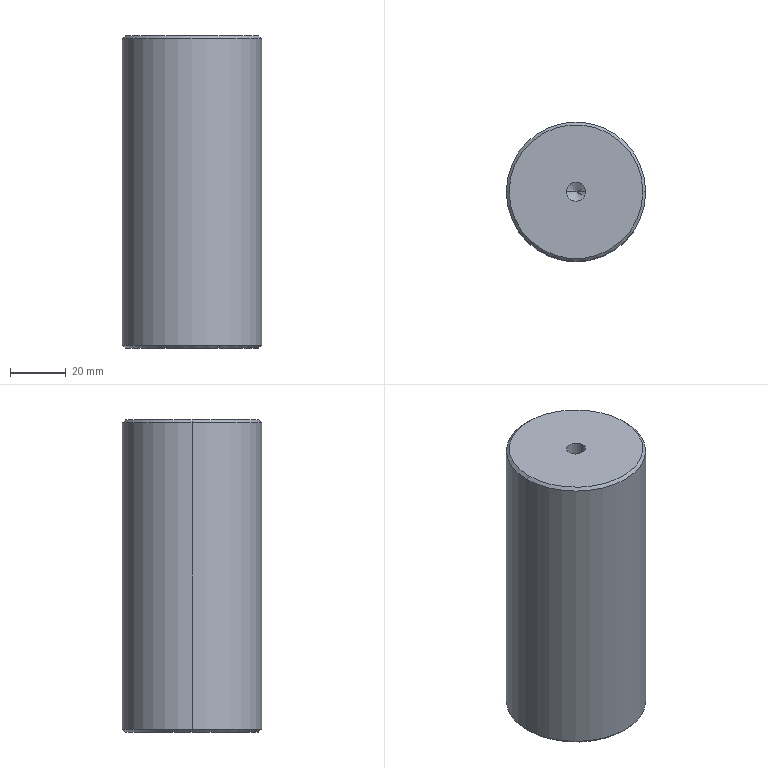Part | SolidWorks | features HoleWzd 2, Chamfer 1, Extrusion 1 | 1 solid | 16 faces | box 50 x 50 x 112 mm | volume 218046 mm3 | cone 8 | cylinder 6 | plane 2 | commonest cylinder face diameters 6.8 x4 50 x2
STEP:
#1=CARTESIAN_POINT('',(24.,0.,112.));
#2=VERTEX_POINT('',#1);
#3=CARTESIAN_POINT('',(-24.,0.,112.));
#4=VERTEX_POINT('',#3);
#5=CARTESIAN_POINT('',(0.,0.,112.));
#6=DIRECTION('',(0.,0.,1.));
#7=DIRECTION('',(1.,0.,0.));
#8=AXIS2_PLACEMENT_3D('',#5,#6,#7);
#9=CIRCLE('',#8,24.);
#10=EDGE_CURVE('',#2,#4,#9,.T.);
#11=ORIENTED_EDGE('',*,*,#10,.F.);
#12=CARTESIAN_POINT('',(25.,0.,111.));
#13=VERTEX_POINT('',#12);
#14=CARTESIAN_POINT('',(24.,0.,112.));
#15=DIRECTION('',(0.7071,0.,-0.7071));
#16=VECTOR('',#15,1000.);
#17=LINE('',#14,#16);
#18=EDGE_CURVE('',#2,#13,#17,.T.);
#19=ORIENTED_EDGE('',*,*,#18,.T.);
#20=CARTESIAN_POINT('',(-25.,0.,111.));
#21=VERTEX_POINT('',#20);
#22=CARTESIAN_POINT('',(0.,0.,111.));
#23=DIRECTION('',(0.,0.,-1.));
#24=DIRECTION('',(1.,0.,0.));
#25=AXIS2_PLACEMENT_3D('',#22,#23,#24);
#26=CIRCLE('',#25,25.);
#27=EDGE_CURVE('',#21,#13,#26,.T.);
#28=ORIENTED_EDGE('',*,*,#27,.F.);
#29=CARTESIAN_POINT('',(-24.,0.,112.));
#30=DIRECTION('',(-0.7071,0.,-0.7071));
#31=VECTOR('',#30,1000.);
#32=LINE('',#29,#31);
#33=EDGE_CURVE('',#4,#21,#32,.T.);
#34=ORIENTED_EDGE('',*,*,#33,.F.);
#35=EDGE_LOOP('',(#11,#19,#28,#34));
#36=FACE_OUTER_BOUND('',#35,.T.);
#37=CARTESIAN_POINT('',(0.,0.,112.));
#38=DIRECTION('',(0.,0.,-1.));
#39=DIRECTION('',(-1.,0.,0.));
#40=AXIS2_PLACEMENT_3D('',#37,#38,#39);
#41=CONICAL_SURFACE('',#40,24.,0.7854);
#42=ADVANCED_FACE('',(#36),#41,.T.);
#43=CARTESIAN_POINT('',(-24.,0.,0.));
#44=VERTEX_POINT('',#43);
#45=CARTESIAN_POINT('',(24.,0.,0.));
#46=VERTEX_POINT('',#45);
#47=CARTESIAN_POINT('',(0.,0.,0.));
#48=DIRECTION('',(0.,0.,-1.));
#49=DIRECTION('',(1.,0.,0.));
#50=AXIS2_PLACEMENT_3D('',#47,#48,#49);
#51=CIRCLE('',#50,24.);
#52=EDGE_CURVE('',#44,#46,#51,.T.);
#53=ORIENTED_EDGE('',*,*,#52,.F.);
#54=CARTESIAN_POINT('',(-25.,0.,1.));
#55=VERTEX_POINT('',#54);
#56=CARTESIAN_POINT('',(-25.,0.,1.));
#57=DIRECTION('',(-0.7071,0.,0.7071));
#58=VECTOR('',#57,1000.);
#59=LINE('',#56,#58);
#60=EDGE_CURVE('',#44,#55,#59,.T.);
#61=ORIENTED_EDGE('',*,*,#60,.T.);
#62=CARTESIAN_POINT('',(25.,0.,1.));
#63=VERTEX_POINT('',#62);
#64=CARTESIAN_POINT('',(0.,0.,1.));
#65=DIRECTION('',(0.,0.,1.));
#66=DIRECTION('',(1.,0.,0.));
#67=AXIS2_PLACEMENT_3D('',#64,#65,#66);
#68=CIRCLE('',#67,25.);
#69=EDGE_CURVE('',#63,#55,#68,.T.);
#70=ORIENTED_EDGE('',*,*,#69,.F.);
#71=CARTESIAN_POINT('',(25.,0.,1.));
#72=DIRECTION('',(0.7071,0.,0.7071));
#73=VECTOR('',#72,1000.);
#74=LINE('',#71,#73);
#75=EDGE_CURVE('',#46,#63,#74,.T.);
#76=ORIENTED_EDGE('',*,*,#75,.F.);
#77=EDGE_LOOP('',(#53,#61,#70,#76));
#78=FACE_OUTER_BOUND('',#77,.T.);
#79=CARTESIAN_POINT('',(0.,0.,1.));
#80=DIRECTION('',(0.,0.,1.));
#81=DIRECTION('',(1.,0.,0.));
#82=AXIS2_PLACEMENT_3D('',#79,#80,#81);
#83=CONICAL_SURFACE('',#82,25.,0.7854);
#84=ADVANCED_FACE('',(#78),#83,.T.);
#85=CARTESIAN_POINT('',(3.4,0.,23.75));
#86=VERTEX_POINT('',#85);
#87=CARTESIAN_POINT('',(-3.4,0.,23.75));
#88=VERTEX_POINT('',#87);
#89=CARTESIAN_POINT('',(0.,0.,23.75));
#90=DIRECTION('',(0.,0.,-1.));
#91=DIRECTION('',(-1.,0.,0.));
#92=AXIS2_PLACEMENT_3D('',#89,#90,#91);
#93=CIRCLE('',#92,3.4);
#94=EDGE_CURVE('',#86,#88,#93,.T.);
#95=ORIENTED_EDGE('',*,*,#94,.F.);
#96=CARTESIAN_POINT('',(3.4,0.,0.));
#97=VERTEX_POINT('',#96);
#98=CARTESIAN_POINT('',(3.4,0.,0.));
#99=DIRECTION('',(0.,0.,-1.));
#100=VECTOR('',#99,1000.);
#101=LINE('',#98,#100);
#102=EDGE_CURVE('',#86,#97,#101,.T.);
#103=ORIENTED_EDGE('',*,*,#102,.T.);
#104=CARTESIAN_POINT('',(-3.4,0.,0.));
#105=VERTEX_POINT('',#104);
#106=CARTESIAN_POINT('',(0.,0.,0.));
#107=DIRECTION('',(0.,0.,-1.));
#108=DIRECTION('',(-1.,0.,0.));
#109=AXIS2_PLACEMENT_3D('',#106,#107,#108);
#110=CIRCLE('',#109,3.4);
#111=EDGE_CURVE('',#97,#105,#110,.T.);
#112=ORIENTED_EDGE('',*,*,#111,.T.);
#113=CARTESIAN_POINT('',(-3.4,0.,0.));
#114=DIRECTION('',(0.,0.,-1.));
#115=VECTOR('',#114,1000.);
#116=LINE('',#113,#115);
#117=EDGE_CURVE('',#88,#105,#116,.T.);
#118=ORIENTED_EDGE('',*,*,#117,.F.);
#119=EDGE_LOOP('',(#95,#103,#112,#118));
#120=FACE_OUTER_BOUND('',#119,.T.);
#121=CARTESIAN_POINT('',(0.,0.,0.));
#122=DIRECTION('',(0.,0.,-1.));
#123=DIRECTION('',(-1.,0.,0.));
#124=AXIS2_PLACEMENT_3D('',#121,#122,#123);
#125=CYLINDRICAL_SURFACE('',#124,3.4);
#126=ADVANCED_FACE('',(#120),#125,.F.);
#127=CARTESIAN_POINT('',(0.,0.,25.793));
#128=VERTEX_POINT('',#127);
#129=CARTESIAN_POINT('',(-3.4,0.,23.75));
#130=DIRECTION('',(-0.8572,0.,-0.515));
#131=VECTOR('',#130,1000.);
#132=LINE('',#129,#131);
#133=EDGE_CURVE('',#128,#88,#132,.T.);
#134=ORIENTED_EDGE('',*,*,#133,.F.);
#135=CARTESIAN_POINT('',(3.4,0.,23.75));
#136=DIRECTION('',(0.8572,0.,-0.515));
#137=VECTOR('',#136,1000.);
#138=LINE('',#135,#137);
#139=EDGE_CURVE('',#128,#86,#138,.T.);
#140=ORIENTED_EDGE('',*,*,#139,.T.);
#141=ORIENTED_EDGE('',*,*,#94,.T.);
#142=EDGE_LOOP('',(#134,#140,#141));
#143=FACE_OUTER_BOUND('',#142,.T.);
#144=CARTESIAN_POINT('',(0.,0.,23.75));
#145=DIRECTION('',(0.,0.,-1.));
#146=DIRECTION('',(-1.,0.,0.));
#147=AXIS2_PLACEMENT_3D('',#144,#145,#146);
#148=CONICAL_SURFACE('',#147,3.4,1.03);
#149=ADVANCED_FACE('',(#143),#148,.F.);
#150=CARTESIAN_POINT('',(-3.4,0.,90.));
#151=VERTEX_POINT('',#150);
#152=CARTESIAN_POINT('',(3.4,0.,90.));
#153=VERTEX_POINT('',#152);
#154=CARTESIAN_POINT('',(0.,0.,90.));
#155=DIRECTION('',(0.,0.,1.));
#156=DIRECTION('',(1.,0.,0.));
#157=AXIS2_PLACEMENT_3D('',#154,#155,#156);
#158=CIRCLE('',#157,3.4);
#159=EDGE_CURVE('',#151,#153,#158,.T.);
#160=ORIENTED_EDGE('',*,*,#159,.F.);
#161=CARTESIAN_POINT('',(-3.4,0.,112.));
#162=VERTEX_POINT('',#161);
#163=CARTESIAN_POINT('',(-3.4,0.,112.));
#164=DIRECTION('',(0.,0.,1.));
#165=VECTOR('',#164,1000.);
#166=LINE('',#163,#165);
#167=EDGE_CURVE('',#151,#162,#166,.T.);
#168=ORIENTED_EDGE('',*,*,#167,.T.);
#169=CARTESIAN_POINT('',(3.4,0.,112.));
#170=VERTEX_POINT('',#169);
#171=CARTESIAN_POINT('',(0.,0.,112.));
#172=DIRECTION('',(0.,0.,1.));
#173=DIRECTION('',(1.,0.,0.));
#174=AXIS2_PLACEMENT_3D('',#171,#172,#173);
#175=CIRCLE('',#174,3.4);
#176=EDGE_CURVE('',#162,#170,#175,.T.);
#177=ORIENTED_EDGE('',*,*,#176,.T.);
#178=CARTESIAN_POINT('',(3.4,0.,112.));
#179=DIRECTION('',(0.,0.,1.));
#180=VECTOR('',#179,1000.);
#181=LINE('',#178,#180);
#182=EDGE_CURVE('',#153,#170,#181,.T.);
#183=ORIENTED_EDGE('',*,*,#182,.F.);
#184=EDGE_LOOP('',(#160,#168,#177,#183));
#185=FACE_OUTER_BOUND('',#184,.T.);
#186=CARTESIAN_POINT('',(0.,0.,112.));
#187=DIRECTION('',(0.,0.,1.));
#188=DIRECTION('',(1.,0.,0.));
#189=AXIS2_PLACEMENT_3D('',#186,#187,#188);
#190=CYLINDRICAL_SURFACE('',#189,3.4);
#191=ADVANCED_FACE('',(#185),#190,.F.);
#192=CARTESIAN_POINT('',(0.,0.,87.957));
#193=VERTEX_POINT('',#192);
#194=CARTESIAN_POINT('',(3.4,0.,90.));
#195=DIRECTION('',(0.8572,0.,0.515));
#196=VECTOR('',#195,1000.);
#197=LINE('',#194,#196);
#198=EDGE_CURVE('',#193,#153,#197,.T.);
#199=ORIENTED_EDGE('',*,*,#198,.F.);
#200=CARTESIAN_POINT('',(-3.4,0.,90.));
#201=DIRECTION('',(-0.8572,0.,0.515));
#202=VECTOR('',#201,1000.);
#203=LINE('',#200,#202);
#204=EDGE_CURVE('',#193,#151,#203,.T.);
#205=ORIENTED_EDGE('',*,*,#204,.T.);
#206=ORIENTED_EDGE('',*,*,#159,.T.);
#207=EDGE_LOOP('',(#199,#205,#206));
#208=FACE_OUTER_BOUND('',#207,.T.);
#209=CARTESIAN_POINT('',(0.,0.,90.));
#210=DIRECTION('',(0.,0.,1.));
#211=DIRECTION('',(1.,0.,0.));
#212=AXIS2_PLACEMENT_3D('',#209,#210,#211);
#213=CONICAL_SURFACE('',#212,3.4,1.03);
#214=ADVANCED_FACE('',(#208),#213,.F.);
#215=ORIENTED_EDGE('',*,*,#27,.T.);
#216=CARTESIAN_POINT('',(25.,0.,112.));
#217=DIRECTION('',(0.,0.,-1.));
#218=VECTOR('',#217,1000.);
#219=LINE('',#216,#218);
#220=EDGE_CURVE('',#13,#63,#219,.T.);
#221=ORIENTED_EDGE('',*,*,#220,.T.);
#222=ORIENTED_EDGE('',*,*,#69,.T.);
#223=CARTESIAN_POINT('',(-25.,0.,112.));
#224=DIRECTION('',(0.,0.,-1.));
#225=VECTOR('',#224,1000.);
#226=LINE('',#223,#225);
#227=EDGE_CURVE('',#21,#55,#226,.T.);
#228=ORIENTED_EDGE('',*,*,#227,.F.);
#229=EDGE_LOOP('',(#215,#221,#222,#228));
#230=FACE_OUTER_BOUND('',#229,.T.);
#231=CARTESIAN_POINT('',(0.,0.,112.));
#232=DIRECTION('',(0.,0.,-1.));
#233=DIRECTION('',(-1.,0.,0.));
#234=AXIS2_PLACEMENT_3D('',#231,#232,#233);
#235=CYLINDRICAL_SURFACE('',#234,25.);
#236=ADVANCED_FACE('',(#230),#235,.T.);
#237=ORIENTED_EDGE('',*,*,#220,.F.);
#238=CARTESIAN_POINT('',(0.,0.,111.));
#239=DIRECTION('',(0.,0.,-1.));
#240=DIRECTION('',(1.,0.,0.));
#241=AXIS2_PLACEMENT_3D('',#238,#239,#240);
#242=CIRCLE('',#241,25.);
#243=EDGE_CURVE('',#13,#21,#242,.T.);
#244=ORIENTED_EDGE('',*,*,#243,.T.);
#245=ORIENTED_EDGE('',*,*,#227,.T.);
#246=CARTESIAN_POINT('',(0.,0.,1.));
#247=DIRECTION('',(0.,0.,1.));
#248=DIRECTION('',(1.,0.,0.));
#249=AXIS2_PLACEMENT_3D('',#246,#247,#248);
#250=CIRCLE('',#249,25.);
#251=EDGE_CURVE('',#55,#63,#250,.T.);
#252=ORIENTED_EDGE('',*,*,#251,.T.);
#253=EDGE_LOOP('',(#237,#244,#245,#252));
#254=FACE_OUTER_BOUND('',#253,.T.);
#255=CARTESIAN_POINT('',(0.,0.,112.));
#256=DIRECTION('',(0.,0.,-1.));
#257=DIRECTION('',(-1.,0.,0.));
#258=AXIS2_PLACEMENT_3D('',#255,#256,#257);
#259=CYLINDRICAL_SURFACE('',#258,25.);
#260=ADVANCED_FACE('',(#254),#259,.T.);
#261=CARTESIAN_POINT('',(0.,0.,112.));
#262=DIRECTION('',(0.,0.,1.));
#263=DIRECTION('',(1.,0.,0.));
#264=AXIS2_PLACEMENT_3D('',#261,#262,#263);
#265=CIRCLE('',#264,24.);
#266=EDGE_CURVE('',#4,#2,#265,.T.);
#267=ORIENTED_EDGE('',*,*,#266,.T.);
#268=ORIENTED_EDGE('',*,*,#10,.T.);
#269=EDGE_LOOP('',(#267,#268));
#270=FACE_OUTER_BOUND('',#269,.T.);
#271=CARTESIAN_POINT('',(0.,0.,112.));
#272=DIRECTION('',(0.,0.,1.));
#273=DIRECTION('',(1.,0.,0.));
#274=AXIS2_PLACEMENT_3D('',#271,#272,#273);
#275=CIRCLE('',#274,3.4);
#276=EDGE_CURVE('',#170,#162,#275,.T.);
#277=ORIENTED_EDGE('',*,*,#276,.F.);
#278=ORIENTED_EDGE('',*,*,#176,.F.);
#279=EDGE_LOOP('',(#277,#278));
#280=FACE_BOUND('',#279,.T.);
#281=CARTESIAN_POINT('',(0.,0.,112.));
#282=DIRECTION('',(0.,0.,1.));
#283=DIRECTION('',(1.,0.,0.));
#284=AXIS2_PLACEMENT_3D('',#281,#282,#283);
#285=PLANE('',#284);
#286=ADVANCED_FACE('',(#270,#280),#285,.T.);
#287=CARTESIAN_POINT('',(0.,0.,0.));
#288=DIRECTION('',(0.,0.,-1.));
#289=DIRECTION('',(1.,0.,0.));
#290=AXIS2_PLACEMENT_3D('',#287,#288,#289);
#291=CIRCLE('',#290,24.);
#292=EDGE_CURVE('',#46,#44,#291,.T.);
#293=ORIENTED_EDGE('',*,*,#292,.T.);
#294=ORIENTED_EDGE('',*,*,#52,.T.);
#295=EDGE_LOOP('',(#293,#294));
#296=FACE_OUTER_BOUND('',#295,.T.);
#297=CARTESIAN_POINT('',(0.,0.,0.));
#298=DIRECTION('',(0.,0.,-1.));
#299=DIRECTION('',(-1.,0.,0.));
#300=AXIS2_PLACEMENT_3D('',#297,#298,#299);
#301=CIRCLE('',#300,3.4);
#302=EDGE_CURVE('',#105,#97,#301,.T.);
#303=ORIENTED_EDGE('',*,*,#302,.F.);
#304=ORIENTED_EDGE('',*,*,#111,.F.);
#305=EDGE_LOOP('',(#303,#304));
#306=FACE_BOUND('',#305,.T.);
#307=CARTESIAN_POINT('',(0.,0.,0.));
#308=DIRECTION('',(0.,0.,1.));
#309=DIRECTION('',(1.,0.,0.));
#310=AXIS2_PLACEMENT_3D('',#307,#308,#309);
#311=PLANE('',#310);
#312=ADVANCED_FACE('',(#296,#306),#311,.F.);
#313=ORIENTED_EDGE('',*,*,#204,.F.);
#314=ORIENTED_EDGE('',*,*,#198,.T.);
#315=CARTESIAN_POINT('',(0.,0.,90.));
#316=DIRECTION('',(0.,0.,1.));
#317=DIRECTION('',(1.,0.,0.));
#318=AXIS2_PLACEMENT_3D('',#315,#316,#317);
#319=CIRCLE('',#318,3.4);
#320=EDGE_CURVE('',#153,#151,#319,.T.);
#321=ORIENTED_EDGE('',*,*,#320,.T.);
#322=EDGE_LOOP('',(#313,#314,#321));
#323=FACE_OUTER_BOUND('',#322,.T.);
#324=CARTESIAN_POINT('',(0.,0.,90.));
#325=DIRECTION('',(0.,0.,1.));
#326=DIRECTION('',(1.,0.,0.));
#327=AXIS2_PLACEMENT_3D('',#324,#325,#326);
#328=CONICAL_SURFACE('',#327,3.4,1.03);
#329=ADVANCED_FACE('',(#323),#328,.F.);
#330=ORIENTED_EDGE('',*,*,#167,.F.);
#331=ORIENTED_EDGE('',*,*,#320,.F.);
#332=ORIENTED_EDGE('',*,*,#182,.T.);
#333=ORIENTED_EDGE('',*,*,#276,.T.);
#334=EDGE_LOOP('',(#330,#331,#332,#333));
#335=FACE_OUTER_BOUND('',#334,.T.);
#336=CARTESIAN_POINT('',(0.,0.,112.));
#337=DIRECTION('',(0.,0.,1.));
#338=DIRECTION('',(1.,0.,0.));
#339=AXIS2_PLACEMENT_3D('',#336,#337,#338);
#340=CYLINDRICAL_SURFACE('',#339,3.4);
#341=ADVANCED_FACE('',(#335),#340,.F.);
#342=ORIENTED_EDGE('',*,*,#139,.F.);
#343=ORIENTED_EDGE('',*,*,#133,.T.);
#344=CARTESIAN_POINT('',(0.,0.,23.75));
#345=DIRECTION('',(0.,0.,-1.));
#346=DIRECTION('',(-1.,0.,0.));
#347=AXIS2_PLACEMENT_3D('',#344,#345,#346);
#348=CIRCLE('',#347,3.4);
#349=EDGE_CURVE('',#88,#86,#348,.T.);
#350=ORIENTED_EDGE('',*,*,#349,.T.);
#351=EDGE_LOOP('',(#342,#343,#350));
#352=FACE_OUTER_BOUND('',#351,.T.);
#353=CARTESIAN_POINT('',(0.,0.,23.75));
#354=DIRECTION('',(0.,0.,-1.));
#355=DIRECTION('',(-1.,0.,0.));
#356=AXIS2_PLACEMENT_3D('',#353,#354,#355);
#357=CONICAL_SURFACE('',#356,3.4,1.03);
#358=ADVANCED_FACE('',(#352),#357,.F.);
#359=ORIENTED_EDGE('',*,*,#102,.F.);
#360=ORIENTED_EDGE('',*,*,#349,.F.);
#361=ORIENTED_EDGE('',*,*,#117,.T.);
#362=ORIENTED_EDGE('',*,*,#302,.T.);
#363=EDGE_LOOP('',(#359,#360,#361,#362));
#364=FACE_OUTER_BOUND('',#363,.T.);
#365=CARTESIAN_POINT('',(0.,0.,0.));
#366=DIRECTION('',(0.,0.,-1.));
#367=DIRECTION('',(-1.,0.,0.));
#368=AXIS2_PLACEMENT_3D('',#365,#366,#367);
#369=CYLINDRICAL_SURFACE('',#368,3.4);
#370=ADVANCED_FACE('',(#364),#369,.F.);
#371=ORIENTED_EDGE('',*,*,#60,.F.);
#372=ORIENTED_EDGE('',*,*,#292,.F.);
#373=ORIENTED_EDGE('',*,*,#75,.T.);
#374=ORIENTED_EDGE('',*,*,#251,.F.);
#375=EDGE_LOOP('',(#371,#372,#373,#374));
#376=FACE_OUTER_BOUND('',#375,.T.);
#377=CARTESIAN_POINT('',(0.,0.,1.));
#378=DIRECTION('',(0.,0.,1.));
#379=DIRECTION('',(1.,0.,0.));
#380=AXIS2_PLACEMENT_3D('',#377,#378,#379);
#381=CONICAL_SURFACE('',#380,25.,0.7854);
#382=ADVANCED_FACE('',(#376),#381,.T.);
#383=ORIENTED_EDGE('',*,*,#18,.F.);
#384=ORIENTED_EDGE('',*,*,#266,.F.);
#385=ORIENTED_EDGE('',*,*,#33,.T.);
#386=ORIENTED_EDGE('',*,*,#243,.F.);
#387=EDGE_LOOP('',(#383,#384,#385,#386));
#388=FACE_OUTER_BOUND('',#387,.T.);
#389=CARTESIAN_POINT('',(0.,0.,112.));
#390=DIRECTION('',(0.,0.,-1.));
#391=DIRECTION('',(-1.,0.,0.));
#392=AXIS2_PLACEMENT_3D('',#389,#390,#391);
#393=CONICAL_SURFACE('',#392,24.,0.7854);
#394=ADVANCED_FACE('',(#388),#393,.T.);
#395=CLOSED_SHELL('',(#42,#84,#126,#149,#191,#214,#236,#260,#286,#312,#329,#341,#358,#370,#382,#394));
#396=MANIFOLD_SOLID_BREP('',#395);
#397=CARTESIAN_POINT('',(0.,0.,0.));
#398=DIRECTION('',(0.,0.,1.));
#399=DIRECTION('',(1.,0.,0.));
#400=AXIS2_PLACEMENT_3D('',#397,#398,#399);
#401=(LENGTH_UNIT()NAMED_UNIT(*)SI_UNIT(.MILLI.,.METRE.));
#402=UNCERTAINTY_MEASURE_WITH_UNIT(LENGTH_MEASURE(0.00001),#401,'','');
#403=(NAMED_UNIT(*)PLANE_ANGLE_UNIT()SI_UNIT($,.RADIAN.));
#404=(NAMED_UNIT(*)SI_UNIT($,.STERADIAN.)SOLID_ANGLE_UNIT());
#405=(GEOMETRIC_REPRESENTATION_CONTEXT(3)GLOBAL_UNCERTAINTY_ASSIGNED_CONTEXT((#402))GLOBAL_UNIT_ASSIGNED_CONTEXT((#401,#403,#404))REPRESENTATION_CONTEXT('',''));
#406=ADVANCED_BREP_SHAPE_REPRESENTATION('',(#396,#400),#405);